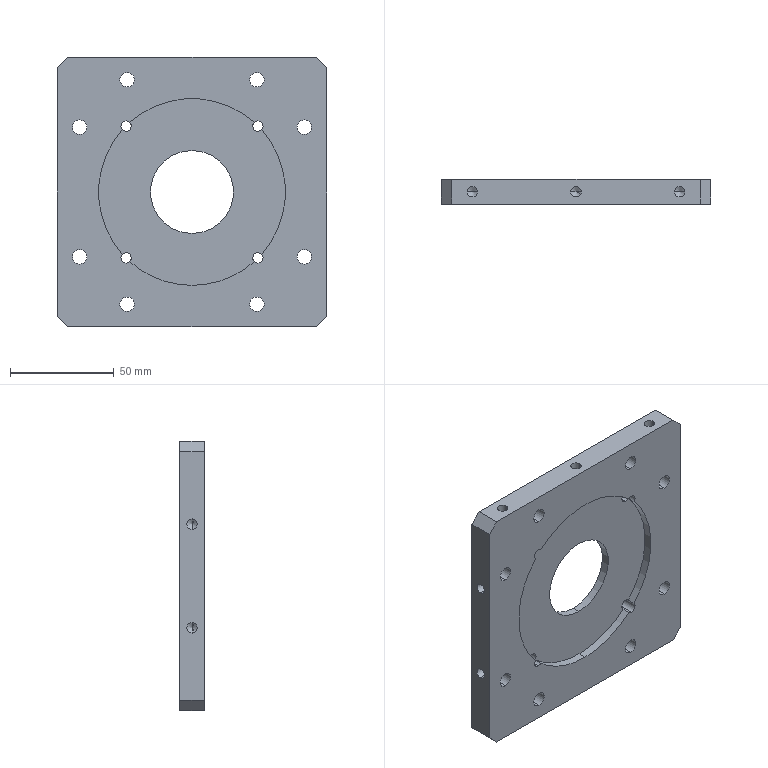Part | SolidWorks | features HoleWzd 6, ICE 2, Chamfer 1, Cut 1, Extrusion 1 | 1 solid | 85 faces | box 130 x 12 x 130 mm | volume 148815 mm3 | cylinder 53 | cone 20 | plane 12 | commonest cylinder face diameters 5 x28 7 x16 90 x5 40 x2 70 x2